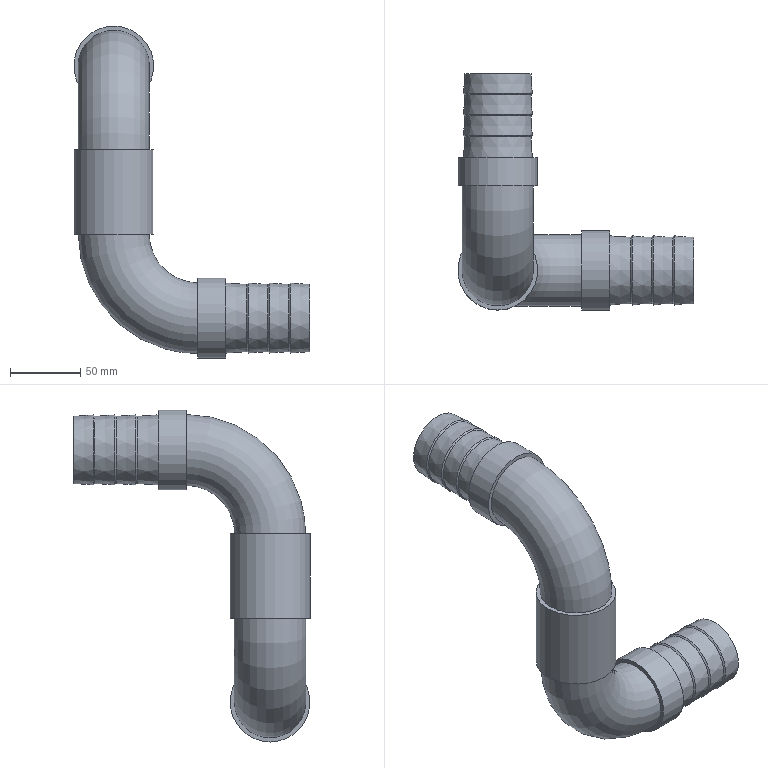Part | STEP file | HL4GZ-1.58.021 (variable pump inlet transition pipe) | 5 solids | 42 faces | box 168.5 x 168.5 x 237 mm | volume 261107 mm3 | cone 20 | plane 12 | cylinder 6 | torus 4 | commonest cylinder face diameters 42 x3 57 x3